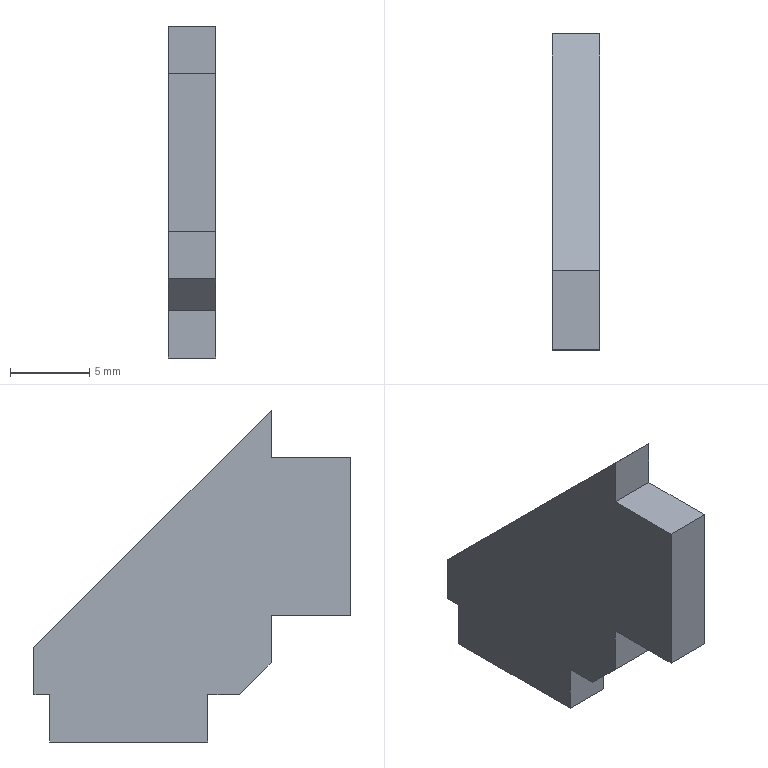Part | SolidWorks | features Chamfer 2, ICE 2, Extrusion 1 | 1 solid | 15 faces | box 3 x 20 x 21 mm | volume 706.5 mm3 | plane 15
STEP:
#1=CARTESIAN_POINT('',(3.,-15.,15.));
#2=VERTEX_POINT('',#1);
#3=CARTESIAN_POINT('',(0.,-15.,15.));
#4=VERTEX_POINT('',#3);
#5=CARTESIAN_POINT('',(0.,-15.,15.));
#6=DIRECTION('',(-1.,0.,0.));
#7=VECTOR('',#6,1000.);
#8=LINE('',#5,#7);
#9=EDGE_CURVE('',#2,#4,#8,.T.);
#10=ORIENTED_EDGE('',*,*,#9,.F.);
#11=CARTESIAN_POINT('',(3.,-15.,18.));
#12=VERTEX_POINT('',#11);
#13=CARTESIAN_POINT('',(3.,-15.,20.));
#14=DIRECTION('',(0.,0.,-1.));
#15=VECTOR('',#14,1000.);
#16=LINE('',#13,#15);
#17=EDGE_CURVE('',#12,#2,#16,.T.);
#18=ORIENTED_EDGE('',*,*,#17,.F.);
#19=CARTESIAN_POINT('',(0.,-15.,18.));
#20=VERTEX_POINT('',#19);
#21=CARTESIAN_POINT('',(0.,-15.,18.));
#22=DIRECTION('',(-1.,0.,0.));
#23=VECTOR('',#22,1000.);
#24=LINE('',#21,#23);
#25=EDGE_CURVE('',#12,#20,#24,.T.);
#26=ORIENTED_EDGE('',*,*,#25,.T.);
#27=CARTESIAN_POINT('',(0.,-15.,20.));
#28=DIRECTION('',(0.,0.,-1.));
#29=VECTOR('',#28,1000.);
#30=LINE('',#27,#29);
#31=EDGE_CURVE('',#20,#4,#30,.T.);
#32=ORIENTED_EDGE('',*,*,#31,.T.);
#33=EDGE_LOOP('',(#10,#18,#26,#32));
#34=FACE_OUTER_BOUND('',#33,.T.);
#35=CARTESIAN_POINT('',(0.,-15.,20.));
#36=DIRECTION('',(0.,1.,0.));
#37=DIRECTION('',(0.,0.,1.));
#38=AXIS2_PLACEMENT_3D('',#35,#36,#37);
#39=PLANE('',#38);
#40=ADVANCED_FACE('',(#34),#39,.F.);
#41=CARTESIAN_POINT('',(0.,-15.,5.));
#42=VERTEX_POINT('',#41);
#43=CARTESIAN_POINT('',(0.,-15.,2.));
#44=VERTEX_POINT('',#43);
#45=CARTESIAN_POINT('',(0.,-15.,20.));
#46=DIRECTION('',(0.,0.,-1.));
#47=VECTOR('',#46,1000.);
#48=LINE('',#45,#47);
#49=EDGE_CURVE('',#42,#44,#48,.T.);
#50=ORIENTED_EDGE('',*,*,#49,.T.);
#51=CARTESIAN_POINT('',(3.,-15.,2.));
#52=VERTEX_POINT('',#51);
#53=CARTESIAN_POINT('',(0.,-15.,2.));
#54=DIRECTION('',(1.,0.,0.));
#55=VECTOR('',#54,1000.);
#56=LINE('',#53,#55);
#57=EDGE_CURVE('',#44,#52,#56,.T.);
#58=ORIENTED_EDGE('',*,*,#57,.T.);
#59=CARTESIAN_POINT('',(3.,-15.,5.));
#60=VERTEX_POINT('',#59);
#61=CARTESIAN_POINT('',(3.,-15.,20.));
#62=DIRECTION('',(0.,0.,-1.));
#63=VECTOR('',#62,1000.);
#64=LINE('',#61,#63);
#65=EDGE_CURVE('',#60,#52,#64,.T.);
#66=ORIENTED_EDGE('',*,*,#65,.F.);
#67=CARTESIAN_POINT('',(0.,-15.,5.));
#68=DIRECTION('',(1.,0.,0.));
#69=VECTOR('',#68,1000.);
#70=LINE('',#67,#69);
#71=EDGE_CURVE('',#42,#60,#70,.T.);
#72=ORIENTED_EDGE('',*,*,#71,.F.);
#73=EDGE_LOOP('',(#50,#58,#66,#72));
#74=FACE_OUTER_BOUND('',#73,.T.);
#75=CARTESIAN_POINT('',(0.,-15.,20.));
#76=DIRECTION('',(0.,1.,0.));
#77=DIRECTION('',(0.,0.,1.));
#78=AXIS2_PLACEMENT_3D('',#75,#76,#77);
#79=PLANE('',#78);
#80=ADVANCED_FACE('',(#74),#79,.F.);
#81=CARTESIAN_POINT('',(0.,-1.,0.));
#82=VERTEX_POINT('',#81);
#83=CARTESIAN_POINT('',(3.,-1.,0.));
#84=VERTEX_POINT('',#83);
#85=CARTESIAN_POINT('',(3.,-1.,0.));
#86=DIRECTION('',(1.,0.,0.));
#87=VECTOR('',#86,1000.);
#88=LINE('',#85,#87);
#89=EDGE_CURVE('',#82,#84,#88,.T.);
#90=ORIENTED_EDGE('',*,*,#89,.F.);
#91=CARTESIAN_POINT('',(0.,0.,0.));
#92=VERTEX_POINT('',#91);
#93=CARTESIAN_POINT('',(0.,0.,0.));
#94=DIRECTION('',(0.,-1.,0.));
#95=VECTOR('',#94,1000.);
#96=LINE('',#93,#95);
#97=EDGE_CURVE('',#92,#82,#96,.T.);
#98=ORIENTED_EDGE('',*,*,#97,.F.);
#99=CARTESIAN_POINT('',(3.,0.,0.));
#100=VERTEX_POINT('',#99);
#101=CARTESIAN_POINT('',(0.,0.,0.));
#102=DIRECTION('',(-1.,0.,0.));
#103=VECTOR('',#102,1000.);
#104=LINE('',#101,#103);
#105=EDGE_CURVE('',#100,#92,#104,.T.);
#106=ORIENTED_EDGE('',*,*,#105,.F.);
#107=CARTESIAN_POINT('',(3.,0.,0.));
#108=DIRECTION('',(0.,1.,0.));
#109=VECTOR('',#108,1000.);
#110=LINE('',#107,#109);
#111=EDGE_CURVE('',#84,#100,#110,.T.);
#112=ORIENTED_EDGE('',*,*,#111,.F.);
#113=EDGE_LOOP('',(#90,#98,#106,#112));
#114=FACE_OUTER_BOUND('',#113,.T.);
#115=CARTESIAN_POINT('',(0.,0.,0.));
#116=DIRECTION('',(0.,0.,1.));
#117=DIRECTION('',(1.,0.,0.));
#118=AXIS2_PLACEMENT_3D('',#115,#116,#117);
#119=PLANE('',#118);
#120=ADVANCED_FACE('',(#114),#119,.F.);
#121=CARTESIAN_POINT('',(3.,-13.,0.));
#122=VERTEX_POINT('',#121);
#123=CARTESIAN_POINT('',(3.,-11.,0.));
#124=VERTEX_POINT('',#123);
#125=CARTESIAN_POINT('',(3.,0.,0.));
#126=DIRECTION('',(0.,1.,0.));
#127=VECTOR('',#126,1000.);
#128=LINE('',#125,#127);
#129=EDGE_CURVE('',#122,#124,#128,.T.);
#130=ORIENTED_EDGE('',*,*,#129,.F.);
#131=CARTESIAN_POINT('',(0.,-13.,0.));
#132=VERTEX_POINT('',#131);
#133=CARTESIAN_POINT('',(0.,-13.,0.));
#134=DIRECTION('',(-1.,0.,0.));
#135=VECTOR('',#134,1000.);
#136=LINE('',#133,#135);
#137=EDGE_CURVE('',#122,#132,#136,.T.);
#138=ORIENTED_EDGE('',*,*,#137,.T.);
#139=CARTESIAN_POINT('',(0.,-11.,0.));
#140=VERTEX_POINT('',#139);
#141=CARTESIAN_POINT('',(0.,0.,0.));
#142=DIRECTION('',(0.,-1.,0.));
#143=VECTOR('',#142,1000.);
#144=LINE('',#141,#143);
#145=EDGE_CURVE('',#140,#132,#144,.T.);
#146=ORIENTED_EDGE('',*,*,#145,.F.);
#147=CARTESIAN_POINT('',(3.,-11.,0.));
#148=DIRECTION('',(-1.,0.,0.));
#149=VECTOR('',#148,1000.);
#150=LINE('',#147,#149);
#151=EDGE_CURVE('',#124,#140,#150,.T.);
#152=ORIENTED_EDGE('',*,*,#151,.F.);
#153=EDGE_LOOP('',(#130,#138,#146,#152));
#154=FACE_OUTER_BOUND('',#153,.T.);
#155=CARTESIAN_POINT('',(0.,0.,0.));
#156=DIRECTION('',(0.,0.,1.));
#157=DIRECTION('',(1.,0.,0.));
#158=AXIS2_PLACEMENT_3D('',#155,#156,#157);
#159=PLANE('',#158);
#160=ADVANCED_FACE('',(#154),#159,.F.);
#161=ORIENTED_EDGE('',*,*,#145,.T.);
#162=CARTESIAN_POINT('',(0.,-15.,2.));
#163=DIRECTION('',(0.,-0.7071,0.7071));
#164=VECTOR('',#163,1000.);
#165=LINE('',#162,#164);
#166=EDGE_CURVE('',#132,#44,#165,.T.);
#167=ORIENTED_EDGE('',*,*,#166,.T.);
#168=ORIENTED_EDGE('',*,*,#49,.F.);
#169=CARTESIAN_POINT('',(0.,-20.,5.));
#170=VERTEX_POINT('',#169);
#171=CARTESIAN_POINT('',(0.,-20.,5.));
#172=DIRECTION('',(0.,1.,0.));
#173=VECTOR('',#172,1000.);
#174=LINE('',#171,#173);
#175=EDGE_CURVE('',#170,#42,#174,.T.);
#176=ORIENTED_EDGE('',*,*,#175,.F.);
#177=CARTESIAN_POINT('',(0.,-20.,15.));
#178=VERTEX_POINT('',#177);
#179=CARTESIAN_POINT('',(0.,-20.,15.));
#180=DIRECTION('',(0.,0.,-1.));
#181=VECTOR('',#180,1000.);
#182=LINE('',#179,#181);
#183=EDGE_CURVE('',#178,#170,#182,.T.);
#184=ORIENTED_EDGE('',*,*,#183,.F.);
#185=CARTESIAN_POINT('',(0.,-20.,15.));
#186=DIRECTION('',(0.,1.,0.));
#187=VECTOR('',#186,1000.);
#188=LINE('',#185,#187);
#189=EDGE_CURVE('',#178,#4,#188,.T.);
#190=ORIENTED_EDGE('',*,*,#189,.T.);
#191=ORIENTED_EDGE('',*,*,#31,.F.);
#192=CARTESIAN_POINT('',(0.,0.,3.));
#193=VERTEX_POINT('',#192);
#194=CARTESIAN_POINT('',(0.,-17.,20.));
#195=DIRECTION('',(0.,0.7071,-0.7071));
#196=VECTOR('',#195,1000.);
#197=LINE('',#194,#196);
#198=EDGE_CURVE('',#20,#193,#197,.T.);
#199=ORIENTED_EDGE('',*,*,#198,.T.);
#200=CARTESIAN_POINT('',(0.,0.,20.));
#201=DIRECTION('',(0.,0.,-1.));
#202=VECTOR('',#201,1000.);
#203=LINE('',#200,#202);
#204=EDGE_CURVE('',#193,#92,#203,.T.);
#205=ORIENTED_EDGE('',*,*,#204,.T.);
#206=ORIENTED_EDGE('',*,*,#97,.T.);
#207=CARTESIAN_POINT('',(0.,-1.,-3.));
#208=VERTEX_POINT('',#207);
#209=CARTESIAN_POINT('',(0.,-1.,-3.));
#210=DIRECTION('',(0.,0.,1.));
#211=VECTOR('',#210,1000.);
#212=LINE('',#209,#211);
#213=EDGE_CURVE('',#208,#82,#212,.T.);
#214=ORIENTED_EDGE('',*,*,#213,.F.);
#215=CARTESIAN_POINT('',(0.,-11.,-3.));
#216=VERTEX_POINT('',#215);
#217=CARTESIAN_POINT('',(0.,-1.,-3.));
#218=DIRECTION('',(0.,1.,0.));
#219=VECTOR('',#218,1000.);
#220=LINE('',#217,#219);
#221=EDGE_CURVE('',#216,#208,#220,.T.);
#222=ORIENTED_EDGE('',*,*,#221,.F.);
#223=CARTESIAN_POINT('',(0.,-11.,-3.));
#224=DIRECTION('',(0.,0.,1.));
#225=VECTOR('',#224,1000.);
#226=LINE('',#223,#225);
#227=EDGE_CURVE('',#216,#140,#226,.T.);
#228=ORIENTED_EDGE('',*,*,#227,.T.);
#229=EDGE_LOOP('',(#161,#167,#168,#176,#184,#190,#191,#199,#205,#206,#214,#222,#228));
#230=FACE_OUTER_BOUND('',#229,.T.);
#231=CARTESIAN_POINT('',(0.,0.,20.));
#232=DIRECTION('',(1.,0.,0.));
#233=DIRECTION('',(0.,1.,0.));
#234=AXIS2_PLACEMENT_3D('',#231,#232,#233);
#235=PLANE('',#234);
#236=ADVANCED_FACE('',(#230),#235,.F.);
#237=ORIENTED_EDGE('',*,*,#65,.T.);
#238=CARTESIAN_POINT('',(3.,-15.,2.));
#239=DIRECTION('',(0.,0.7071,-0.7071));
#240=VECTOR('',#239,1000.);
#241=LINE('',#238,#240);
#242=EDGE_CURVE('',#52,#122,#241,.T.);
#243=ORIENTED_EDGE('',*,*,#242,.T.);
#244=ORIENTED_EDGE('',*,*,#129,.T.);
#245=CARTESIAN_POINT('',(3.,-11.,-3.));
#246=VERTEX_POINT('',#245);
#247=CARTESIAN_POINT('',(3.,-11.,-3.));
#248=DIRECTION('',(0.,0.,1.));
#249=VECTOR('',#248,1000.);
#250=LINE('',#247,#249);
#251=EDGE_CURVE('',#246,#124,#250,.T.);
#252=ORIENTED_EDGE('',*,*,#251,.F.);
#253=CARTESIAN_POINT('',(3.,-1.,-3.));
#254=VERTEX_POINT('',#253);
#255=CARTESIAN_POINT('',(3.,-1.,-3.));
#256=DIRECTION('',(0.,-1.,0.));
#257=VECTOR('',#256,1000.);
#258=LINE('',#255,#257);
#259=EDGE_CURVE('',#254,#246,#258,.T.);
#260=ORIENTED_EDGE('',*,*,#259,.F.);
#261=CARTESIAN_POINT('',(3.,-1.,-3.));
#262=DIRECTION('',(0.,0.,1.));
#263=VECTOR('',#262,1000.);
#264=LINE('',#261,#263);
#265=EDGE_CURVE('',#254,#84,#264,.T.);
#266=ORIENTED_EDGE('',*,*,#265,.T.);
#267=ORIENTED_EDGE('',*,*,#111,.T.);
#268=CARTESIAN_POINT('',(3.,0.,3.));
#269=VERTEX_POINT('',#268);
#270=CARTESIAN_POINT('',(3.,0.,20.));
#271=DIRECTION('',(0.,0.,-1.));
#272=VECTOR('',#271,1000.);
#273=LINE('',#270,#272);
#274=EDGE_CURVE('',#269,#100,#273,.T.);
#275=ORIENTED_EDGE('',*,*,#274,.F.);
#276=CARTESIAN_POINT('',(3.,-17.,20.));
#277=DIRECTION('',(0.,-0.7071,0.7071));
#278=VECTOR('',#277,1000.);
#279=LINE('',#276,#278);
#280=EDGE_CURVE('',#269,#12,#279,.T.);
#281=ORIENTED_EDGE('',*,*,#280,.T.);
#282=ORIENTED_EDGE('',*,*,#17,.T.);
#283=CARTESIAN_POINT('',(3.,-20.,15.));
#284=VERTEX_POINT('',#283);
#285=CARTESIAN_POINT('',(3.,-20.,15.));
#286=DIRECTION('',(0.,1.,0.));
#287=VECTOR('',#286,1000.);
#288=LINE('',#285,#287);
#289=EDGE_CURVE('',#284,#2,#288,.T.);
#290=ORIENTED_EDGE('',*,*,#289,.F.);
#291=CARTESIAN_POINT('',(3.,-20.,5.));
#292=VERTEX_POINT('',#291);
#293=CARTESIAN_POINT('',(3.,-20.,15.));
#294=DIRECTION('',(0.,0.,1.));
#295=VECTOR('',#294,1000.);
#296=LINE('',#293,#295);
#297=EDGE_CURVE('',#292,#284,#296,.T.);
#298=ORIENTED_EDGE('',*,*,#297,.F.);
#299=CARTESIAN_POINT('',(3.,-20.,5.));
#300=DIRECTION('',(0.,1.,0.));
#301=VECTOR('',#300,1000.);
#302=LINE('',#299,#301);
#303=EDGE_CURVE('',#292,#60,#302,.T.);
#304=ORIENTED_EDGE('',*,*,#303,.T.);
#305=EDGE_LOOP('',(#237,#243,#244,#252,#260,#266,#267,#275,#281,#282,#290,#298,#304));
#306=FACE_OUTER_BOUND('',#305,.T.);
#307=CARTESIAN_POINT('',(3.,0.,20.));
#308=DIRECTION('',(-1.,0.,0.));
#309=DIRECTION('',(0.,-1.,0.));
#310=AXIS2_PLACEMENT_3D('',#307,#308,#309);
#311=PLANE('',#310);
#312=ADVANCED_FACE('',(#306),#311,.F.);
#313=ORIENTED_EDGE('',*,*,#204,.F.);
#314=CARTESIAN_POINT('',(3.,0.,3.));
#315=DIRECTION('',(1.,0.,0.));
#316=VECTOR('',#315,1000.);
#317=LINE('',#314,#316);
#318=EDGE_CURVE('',#193,#269,#317,.T.);
#319=ORIENTED_EDGE('',*,*,#318,.T.);
#320=ORIENTED_EDGE('',*,*,#274,.T.);
#321=ORIENTED_EDGE('',*,*,#105,.T.);
#322=EDGE_LOOP('',(#313,#319,#320,#321));
#323=FACE_OUTER_BOUND('',#322,.T.);
#324=CARTESIAN_POINT('',(0.,0.,20.));
#325=DIRECTION('',(0.,-1.,0.));
#326=DIRECTION('',(0.,0.,-1.));
#327=AXIS2_PLACEMENT_3D('',#324,#325,#326);
#328=PLANE('',#327);
#329=ADVANCED_FACE('',(#323),#328,.F.);
#330=ORIENTED_EDGE('',*,*,#151,.T.);
#331=ORIENTED_EDGE('',*,*,#227,.F.);
#332=CARTESIAN_POINT('',(3.,-11.,-3.));
#333=DIRECTION('',(-1.,0.,0.));
#334=VECTOR('',#333,1000.);
#335=LINE('',#332,#334);
#336=EDGE_CURVE('',#246,#216,#335,.T.);
#337=ORIENTED_EDGE('',*,*,#336,.F.);
#338=ORIENTED_EDGE('',*,*,#251,.T.);
#339=EDGE_LOOP('',(#330,#331,#337,#338));
#340=FACE_OUTER_BOUND('',#339,.T.);
#341=CARTESIAN_POINT('',(3.,-11.,-3.));
#342=DIRECTION('',(0.,1.,0.));
#343=DIRECTION('',(0.,0.,1.));
#344=AXIS2_PLACEMENT_3D('',#341,#342,#343);
#345=PLANE('',#344);
#346=ADVANCED_FACE('',(#340),#345,.F.);
#347=ORIENTED_EDGE('',*,*,#89,.T.);
#348=ORIENTED_EDGE('',*,*,#265,.F.);
#349=CARTESIAN_POINT('',(3.,-1.,-3.));
#350=DIRECTION('',(1.,0.,0.));
#351=VECTOR('',#350,1000.);
#352=LINE('',#349,#351);
#353=EDGE_CURVE('',#208,#254,#352,.T.);
#354=ORIENTED_EDGE('',*,*,#353,.F.);
#355=ORIENTED_EDGE('',*,*,#213,.T.);
#356=EDGE_LOOP('',(#347,#348,#354,#355));
#357=FACE_OUTER_BOUND('',#356,.T.);
#358=CARTESIAN_POINT('',(3.,-1.,-3.));
#359=DIRECTION('',(0.,-1.,0.));
#360=DIRECTION('',(0.,0.,-1.));
#361=AXIS2_PLACEMENT_3D('',#358,#359,#360);
#362=PLANE('',#361);
#363=ADVANCED_FACE('',(#357),#362,.F.);
#364=ORIENTED_EDGE('',*,*,#259,.T.);
#365=ORIENTED_EDGE('',*,*,#336,.T.);
#366=ORIENTED_EDGE('',*,*,#221,.T.);
#367=ORIENTED_EDGE('',*,*,#353,.T.);
#368=EDGE_LOOP('',(#364,#365,#366,#367));
#369=FACE_OUTER_BOUND('',#368,.T.);
#370=CARTESIAN_POINT('',(0.,0.,-3.));
#371=DIRECTION('',(0.,0.,-1.));
#372=DIRECTION('',(-1.,0.,0.));
#373=AXIS2_PLACEMENT_3D('',#370,#371,#372);
#374=PLANE('',#373);
#375=ADVANCED_FACE('',(#369),#374,.T.);
#376=ORIENTED_EDGE('',*,*,#280,.F.);
#377=ORIENTED_EDGE('',*,*,#318,.F.);
#378=ORIENTED_EDGE('',*,*,#198,.F.);
#379=ORIENTED_EDGE('',*,*,#25,.F.);
#380=EDGE_LOOP('',(#376,#377,#378,#379));
#381=FACE_OUTER_BOUND('',#380,.T.);
#382=CARTESIAN_POINT('',(0.,-17.,20.));
#383=DIRECTION('',(0.,0.7071,0.7071));
#384=DIRECTION('',(1.,0.,0.));
#385=AXIS2_PLACEMENT_3D('',#382,#383,#384);
#386=PLANE('',#385);
#387=ADVANCED_FACE('',(#381),#386,.T.);
#388=ORIENTED_EDGE('',*,*,#71,.T.);
#389=ORIENTED_EDGE('',*,*,#303,.F.);
#390=CARTESIAN_POINT('',(0.,-20.,5.));
#391=DIRECTION('',(1.,0.,0.));
#392=VECTOR('',#391,1000.);
#393=LINE('',#390,#392);
#394=EDGE_CURVE('',#170,#292,#393,.T.);
#395=ORIENTED_EDGE('',*,*,#394,.F.);
#396=ORIENTED_EDGE('',*,*,#175,.T.);
#397=EDGE_LOOP('',(#388,#389,#395,#396));
#398=FACE_OUTER_BOUND('',#397,.T.);
#399=CARTESIAN_POINT('',(0.,-20.,5.));
#400=DIRECTION('',(0.,0.,1.));
#401=DIRECTION('',(1.,0.,0.));
#402=AXIS2_PLACEMENT_3D('',#399,#400,#401);
#403=PLANE('',#402);
#404=ADVANCED_FACE('',(#398),#403,.F.);
#405=ORIENTED_EDGE('',*,*,#9,.T.);
#406=ORIENTED_EDGE('',*,*,#189,.F.);
#407=CARTESIAN_POINT('',(0.,-20.,15.));
#408=DIRECTION('',(-1.,0.,0.));
#409=VECTOR('',#408,1000.);
#410=LINE('',#407,#409);
#411=EDGE_CURVE('',#284,#178,#410,.T.);
#412=ORIENTED_EDGE('',*,*,#411,.F.);
#413=ORIENTED_EDGE('',*,*,#289,.T.);
#414=EDGE_LOOP('',(#405,#406,#412,#413));
#415=FACE_OUTER_BOUND('',#414,.T.);
#416=CARTESIAN_POINT('',(0.,-20.,15.));
#417=DIRECTION('',(0.,0.,-1.));
#418=DIRECTION('',(-1.,0.,0.));
#419=AXIS2_PLACEMENT_3D('',#416,#417,#418);
#420=PLANE('',#419);
#421=ADVANCED_FACE('',(#415),#420,.F.);
#422=ORIENTED_EDGE('',*,*,#183,.T.);
#423=ORIENTED_EDGE('',*,*,#394,.T.);
#424=ORIENTED_EDGE('',*,*,#297,.T.);
#425=ORIENTED_EDGE('',*,*,#411,.T.);
#426=EDGE_LOOP('',(#422,#423,#424,#425));
#427=FACE_OUTER_BOUND('',#426,.T.);
#428=CARTESIAN_POINT('',(0.,-20.,0.));
#429=DIRECTION('',(0.,-1.,0.));
#430=DIRECTION('',(0.,0.,-1.));
#431=AXIS2_PLACEMENT_3D('',#428,#429,#430);
#432=PLANE('',#431);
#433=ADVANCED_FACE('',(#427),#432,.T.);
#434=ORIENTED_EDGE('',*,*,#166,.F.);
#435=ORIENTED_EDGE('',*,*,#137,.F.);
#436=ORIENTED_EDGE('',*,*,#242,.F.);
#437=ORIENTED_EDGE('',*,*,#57,.F.);
#438=EDGE_LOOP('',(#434,#435,#436,#437));
#439=FACE_OUTER_BOUND('',#438,.T.);
#440=CARTESIAN_POINT('',(0.,-15.,2.));
#441=DIRECTION('',(0.,0.7071,0.7071));
#442=DIRECTION('',(1.,0.,0.));
#443=AXIS2_PLACEMENT_3D('',#440,#441,#442);
#444=PLANE('',#443);
#445=ADVANCED_FACE('',(#439),#444,.F.);
#446=CLOSED_SHELL('',(#40,#80,#120,#160,#236,#312,#329,#346,#363,#375,#387,#404,#421,#433,#445));
#447=MANIFOLD_SOLID_BREP('',#446);
#448=CARTESIAN_POINT('',(0.,0.,0.));
#449=DIRECTION('',(0.,0.,1.));
#450=DIRECTION('',(1.,0.,0.));
#451=AXIS2_PLACEMENT_3D('',#448,#449,#450);
#452=(LENGTH_UNIT()NAMED_UNIT(*)SI_UNIT(.MILLI.,.METRE.));
#453=UNCERTAINTY_MEASURE_WITH_UNIT(LENGTH_MEASURE(0.00001),#452,'','');
#454=(NAMED_UNIT(*)PLANE_ANGLE_UNIT()SI_UNIT($,.RADIAN.));
#455=(NAMED_UNIT(*)SI_UNIT($,.STERADIAN.)SOLID_ANGLE_UNIT());
#456=(GEOMETRIC_REPRESENTATION_CONTEXT(3)GLOBAL_UNCERTAINTY_ASSIGNED_CONTEXT((#453))GLOBAL_UNIT_ASSIGNED_CONTEXT((#452,#454,#455))REPRESENTATION_CONTEXT('',''));
#457=ADVANCED_BREP_SHAPE_REPRESENTATION('',(#447,#451),#456);